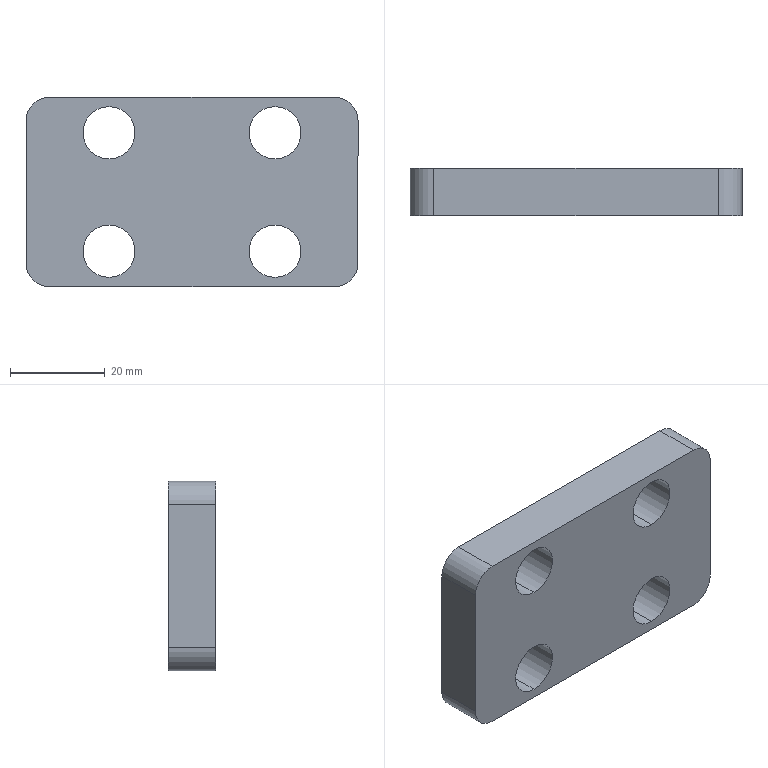Part | SolidWorks | features Extrusion 1, Fillet 1, HoleWzd 1 | 1 solid | 18 faces | box 70 x 10 x 40 mm | volume 23984 mm3 | cylinder 12 | plane 6 | commonest cylinder face diameters 11 x8 10 x4
STEP:
#1=CARTESIAN_POINT('',(-17.5,-5.,-18.));
#2=VERTEX_POINT('',#1);
#3=CARTESIAN_POINT('',(-17.5,-5.,-7.));
#4=VERTEX_POINT('',#3);
#5=CARTESIAN_POINT('',(-17.5,-5.,-12.5));
#6=DIRECTION('',(0.,1.,0.));
#7=DIRECTION('',(0.,0.,1.));
#8=AXIS2_PLACEMENT_3D('',#5,#6,#7);
#9=CIRCLE('',#8,5.5);
#10=EDGE_CURVE('',#2,#4,#9,.T.);
#11=ORIENTED_EDGE('',*,*,#10,.F.);
#12=CARTESIAN_POINT('',(-17.5,5.,-18.));
#13=VERTEX_POINT('',#12);
#14=CARTESIAN_POINT('',(-17.5,5.,-18.));
#15=DIRECTION('',(0.,1.,0.));
#16=VECTOR('',#15,1000.);
#17=LINE('',#14,#16);
#18=EDGE_CURVE('',#2,#13,#17,.T.);
#19=ORIENTED_EDGE('',*,*,#18,.T.);
#20=CARTESIAN_POINT('',(-17.5,5.,-7.));
#21=VERTEX_POINT('',#20);
#22=CARTESIAN_POINT('',(-17.5,5.,-12.5));
#23=DIRECTION('',(0.,1.,0.));
#24=DIRECTION('',(0.,0.,1.));
#25=AXIS2_PLACEMENT_3D('',#22,#23,#24);
#26=CIRCLE('',#25,5.5);
#27=EDGE_CURVE('',#13,#21,#26,.T.);
#28=ORIENTED_EDGE('',*,*,#27,.T.);
#29=CARTESIAN_POINT('',(-17.5,5.,-7.));
#30=DIRECTION('',(0.,1.,0.));
#31=VECTOR('',#30,1000.);
#32=LINE('',#29,#31);
#33=EDGE_CURVE('',#4,#21,#32,.T.);
#34=ORIENTED_EDGE('',*,*,#33,.F.);
#35=EDGE_LOOP('',(#11,#19,#28,#34));
#36=FACE_OUTER_BOUND('',#35,.T.);
#37=CARTESIAN_POINT('',(-17.5,5.,-12.5));
#38=DIRECTION('',(0.,1.,0.));
#39=DIRECTION('',(0.,0.,1.));
#40=AXIS2_PLACEMENT_3D('',#37,#38,#39);
#41=CYLINDRICAL_SURFACE('',#40,5.5);
#42=ADVANCED_FACE('',(#36),#41,.F.);
#43=CARTESIAN_POINT('',(17.5,-5.,-18.));
#44=VERTEX_POINT('',#43);
#45=CARTESIAN_POINT('',(17.5,-5.,-7.));
#46=VERTEX_POINT('',#45);
#47=CARTESIAN_POINT('',(17.5,-5.,-12.5));
#48=DIRECTION('',(0.,1.,0.));
#49=DIRECTION('',(0.,0.,1.));
#50=AXIS2_PLACEMENT_3D('',#47,#48,#49);
#51=CIRCLE('',#50,5.5);
#52=EDGE_CURVE('',#44,#46,#51,.T.);
#53=ORIENTED_EDGE('',*,*,#52,.F.);
#54=CARTESIAN_POINT('',(17.5,5.,-18.));
#55=VERTEX_POINT('',#54);
#56=CARTESIAN_POINT('',(17.5,5.,-18.));
#57=DIRECTION('',(0.,1.,0.));
#58=VECTOR('',#57,1000.);
#59=LINE('',#56,#58);
#60=EDGE_CURVE('',#44,#55,#59,.T.);
#61=ORIENTED_EDGE('',*,*,#60,.T.);
#62=CARTESIAN_POINT('',(17.5,5.,-7.));
#63=VERTEX_POINT('',#62);
#64=CARTESIAN_POINT('',(17.5,5.,-12.5));
#65=DIRECTION('',(0.,1.,0.));
#66=DIRECTION('',(0.,0.,1.));
#67=AXIS2_PLACEMENT_3D('',#64,#65,#66);
#68=CIRCLE('',#67,5.5);
#69=EDGE_CURVE('',#55,#63,#68,.T.);
#70=ORIENTED_EDGE('',*,*,#69,.T.);
#71=CARTESIAN_POINT('',(17.5,5.,-7.));
#72=DIRECTION('',(0.,1.,0.));
#73=VECTOR('',#72,1000.);
#74=LINE('',#71,#73);
#75=EDGE_CURVE('',#46,#63,#74,.T.);
#76=ORIENTED_EDGE('',*,*,#75,.F.);
#77=EDGE_LOOP('',(#53,#61,#70,#76));
#78=FACE_OUTER_BOUND('',#77,.T.);
#79=CARTESIAN_POINT('',(17.5,5.,-12.5));
#80=DIRECTION('',(0.,1.,0.));
#81=DIRECTION('',(0.,0.,1.));
#82=AXIS2_PLACEMENT_3D('',#79,#80,#81);
#83=CYLINDRICAL_SURFACE('',#82,5.5);
#84=ADVANCED_FACE('',(#78),#83,.F.);
#85=CARTESIAN_POINT('',(17.5,-5.,7.));
#86=VERTEX_POINT('',#85);
#87=CARTESIAN_POINT('',(17.5,-5.,18.));
#88=VERTEX_POINT('',#87);
#89=CARTESIAN_POINT('',(17.5,-5.,12.5));
#90=DIRECTION('',(0.,1.,0.));
#91=DIRECTION('',(0.,0.,1.));
#92=AXIS2_PLACEMENT_3D('',#89,#90,#91);
#93=CIRCLE('',#92,5.5);
#94=EDGE_CURVE('',#86,#88,#93,.T.);
#95=ORIENTED_EDGE('',*,*,#94,.F.);
#96=CARTESIAN_POINT('',(17.5,5.,7.));
#97=VERTEX_POINT('',#96);
#98=CARTESIAN_POINT('',(17.5,5.,7.));
#99=DIRECTION('',(0.,1.,0.));
#100=VECTOR('',#99,1000.);
#101=LINE('',#98,#100);
#102=EDGE_CURVE('',#86,#97,#101,.T.);
#103=ORIENTED_EDGE('',*,*,#102,.T.);
#104=CARTESIAN_POINT('',(17.5,5.,18.));
#105=VERTEX_POINT('',#104);
#106=CARTESIAN_POINT('',(17.5,5.,12.5));
#107=DIRECTION('',(0.,1.,0.));
#108=DIRECTION('',(0.,0.,1.));
#109=AXIS2_PLACEMENT_3D('',#106,#107,#108);
#110=CIRCLE('',#109,5.5);
#111=EDGE_CURVE('',#97,#105,#110,.T.);
#112=ORIENTED_EDGE('',*,*,#111,.T.);
#113=CARTESIAN_POINT('',(17.5,5.,18.));
#114=DIRECTION('',(0.,1.,0.));
#115=VECTOR('',#114,1000.);
#116=LINE('',#113,#115);
#117=EDGE_CURVE('',#88,#105,#116,.T.);
#118=ORIENTED_EDGE('',*,*,#117,.F.);
#119=EDGE_LOOP('',(#95,#103,#112,#118));
#120=FACE_OUTER_BOUND('',#119,.T.);
#121=CARTESIAN_POINT('',(17.5,5.,12.5));
#122=DIRECTION('',(0.,1.,0.));
#123=DIRECTION('',(0.,0.,1.));
#124=AXIS2_PLACEMENT_3D('',#121,#122,#123);
#125=CYLINDRICAL_SURFACE('',#124,5.5);
#126=ADVANCED_FACE('',(#120),#125,.F.);
#127=CARTESIAN_POINT('',(-17.5,-5.,7.));
#128=VERTEX_POINT('',#127);
#129=CARTESIAN_POINT('',(-17.5,-5.,18.));
#130=VERTEX_POINT('',#129);
#131=CARTESIAN_POINT('',(-17.5,-5.,12.5));
#132=DIRECTION('',(0.,1.,0.));
#133=DIRECTION('',(0.,0.,1.));
#134=AXIS2_PLACEMENT_3D('',#131,#132,#133);
#135=CIRCLE('',#134,5.5);
#136=EDGE_CURVE('',#128,#130,#135,.T.);
#137=ORIENTED_EDGE('',*,*,#136,.F.);
#138=CARTESIAN_POINT('',(-17.5,5.,7.));
#139=VERTEX_POINT('',#138);
#140=CARTESIAN_POINT('',(-17.5,5.,7.));
#141=DIRECTION('',(0.,1.,0.));
#142=VECTOR('',#141,1000.);
#143=LINE('',#140,#142);
#144=EDGE_CURVE('',#128,#139,#143,.T.);
#145=ORIENTED_EDGE('',*,*,#144,.T.);
#146=CARTESIAN_POINT('',(-17.5,5.,18.));
#147=VERTEX_POINT('',#146);
#148=CARTESIAN_POINT('',(-17.5,5.,12.5));
#149=DIRECTION('',(0.,1.,0.));
#150=DIRECTION('',(0.,0.,1.));
#151=AXIS2_PLACEMENT_3D('',#148,#149,#150);
#152=CIRCLE('',#151,5.5);
#153=EDGE_CURVE('',#139,#147,#152,.T.);
#154=ORIENTED_EDGE('',*,*,#153,.T.);
#155=CARTESIAN_POINT('',(-17.5,5.,18.));
#156=DIRECTION('',(0.,1.,0.));
#157=VECTOR('',#156,1000.);
#158=LINE('',#155,#157);
#159=EDGE_CURVE('',#130,#147,#158,.T.);
#160=ORIENTED_EDGE('',*,*,#159,.F.);
#161=EDGE_LOOP('',(#137,#145,#154,#160));
#162=FACE_OUTER_BOUND('',#161,.T.);
#163=CARTESIAN_POINT('',(-17.5,5.,12.5));
#164=DIRECTION('',(0.,1.,0.));
#165=DIRECTION('',(0.,0.,1.));
#166=AXIS2_PLACEMENT_3D('',#163,#164,#165);
#167=CYLINDRICAL_SURFACE('',#166,5.5);
#168=ADVANCED_FACE('',(#162),#167,.F.);
#169=CARTESIAN_POINT('',(35.,5.,15.));
#170=VERTEX_POINT('',#169);
#171=CARTESIAN_POINT('',(35.,5.,-15.));
#172=VERTEX_POINT('',#171);
#173=CARTESIAN_POINT('',(35.,5.,-20.));
#174=DIRECTION('',(0.,0.,-1.));
#175=VECTOR('',#174,1000.);
#176=LINE('',#173,#175);
#177=EDGE_CURVE('',#170,#172,#176,.T.);
#178=ORIENTED_EDGE('',*,*,#177,.F.);
#179=CARTESIAN_POINT('',(35.,-5.,15.));
#180=VERTEX_POINT('',#179);
#181=CARTESIAN_POINT('',(35.,5.,15.));
#182=DIRECTION('',(0.,-1.,0.));
#183=VECTOR('',#182,1000.);
#184=LINE('',#181,#183);
#185=EDGE_CURVE('',#170,#180,#184,.T.);
#186=ORIENTED_EDGE('',*,*,#185,.T.);
#187=CARTESIAN_POINT('',(35.,-5.,-15.));
#188=VERTEX_POINT('',#187);
#189=CARTESIAN_POINT('',(35.,-5.,-20.));
#190=DIRECTION('',(0.,0.,-1.));
#191=VECTOR('',#190,1000.);
#192=LINE('',#189,#191);
#193=EDGE_CURVE('',#180,#188,#192,.T.);
#194=ORIENTED_EDGE('',*,*,#193,.T.);
#195=CARTESIAN_POINT('',(35.,5.,-15.));
#196=DIRECTION('',(0.,1.,0.));
#197=VECTOR('',#196,1000.);
#198=LINE('',#195,#197);
#199=EDGE_CURVE('',#188,#172,#198,.T.);
#200=ORIENTED_EDGE('',*,*,#199,.T.);
#201=EDGE_LOOP('',(#178,#186,#194,#200));
#202=FACE_OUTER_BOUND('',#201,.T.);
#203=CARTESIAN_POINT('',(35.,5.,-20.));
#204=DIRECTION('',(-1.,0.,0.));
#205=DIRECTION('',(0.,0.,1.));
#206=AXIS2_PLACEMENT_3D('',#203,#204,#205);
#207=PLANE('',#206);
#208=ADVANCED_FACE('',(#202),#207,.F.);
#209=CARTESIAN_POINT('',(30.,-5.,-20.));
#210=VERTEX_POINT('',#209);
#211=CARTESIAN_POINT('',(-30.,-5.,-20.));
#212=VERTEX_POINT('',#211);
#213=CARTESIAN_POINT('',(-35.,-5.,-20.));
#214=DIRECTION('',(-1.,0.,0.));
#215=VECTOR('',#214,1000.);
#216=LINE('',#213,#215);
#217=EDGE_CURVE('',#210,#212,#216,.T.);
#218=ORIENTED_EDGE('',*,*,#217,.T.);
#219=CARTESIAN_POINT('',(-30.,5.,-20.));
#220=VERTEX_POINT('',#219);
#221=CARTESIAN_POINT('',(-30.,5.,-20.));
#222=DIRECTION('',(0.,1.,0.));
#223=VECTOR('',#222,1000.);
#224=LINE('',#221,#223);
#225=EDGE_CURVE('',#212,#220,#224,.T.);
#226=ORIENTED_EDGE('',*,*,#225,.T.);
#227=CARTESIAN_POINT('',(30.,5.,-20.));
#228=VERTEX_POINT('',#227);
#229=CARTESIAN_POINT('',(-35.,5.,-20.));
#230=DIRECTION('',(-1.,0.,0.));
#231=VECTOR('',#230,1000.);
#232=LINE('',#229,#231);
#233=EDGE_CURVE('',#228,#220,#232,.T.);
#234=ORIENTED_EDGE('',*,*,#233,.F.);
#235=CARTESIAN_POINT('',(30.,5.,-20.));
#236=DIRECTION('',(0.,-1.,0.));
#237=VECTOR('',#236,1000.);
#238=LINE('',#235,#237);
#239=EDGE_CURVE('',#228,#210,#238,.T.);
#240=ORIENTED_EDGE('',*,*,#239,.T.);
#241=EDGE_LOOP('',(#218,#226,#234,#240));
#242=FACE_OUTER_BOUND('',#241,.T.);
#243=CARTESIAN_POINT('',(-35.,5.,-20.));
#244=DIRECTION('',(0.,0.,1.));
#245=DIRECTION('',(1.,0.,0.));
#246=AXIS2_PLACEMENT_3D('',#243,#244,#245);
#247=PLANE('',#246);
#248=ADVANCED_FACE('',(#242),#247,.F.);
#249=CARTESIAN_POINT('',(-35.,5.,-15.));
#250=VERTEX_POINT('',#249);
#251=CARTESIAN_POINT('',(-35.,5.,15.));
#252=VERTEX_POINT('',#251);
#253=CARTESIAN_POINT('',(-35.,5.,-20.));
#254=DIRECTION('',(0.,0.,1.));
#255=VECTOR('',#254,1000.);
#256=LINE('',#253,#255);
#257=EDGE_CURVE('',#250,#252,#256,.T.);
#258=ORIENTED_EDGE('',*,*,#257,.F.);
#259=CARTESIAN_POINT('',(-35.,-5.,-15.));
#260=VERTEX_POINT('',#259);
#261=CARTESIAN_POINT('',(-35.,5.,-15.));
#262=DIRECTION('',(0.,-1.,0.));
#263=VECTOR('',#262,1000.);
#264=LINE('',#261,#263);
#265=EDGE_CURVE('',#250,#260,#264,.T.);
#266=ORIENTED_EDGE('',*,*,#265,.T.);
#267=CARTESIAN_POINT('',(-35.,-5.,15.));
#268=VERTEX_POINT('',#267);
#269=CARTESIAN_POINT('',(-35.,-5.,-20.));
#270=DIRECTION('',(0.,0.,1.));
#271=VECTOR('',#270,1000.);
#272=LINE('',#269,#271);
#273=EDGE_CURVE('',#260,#268,#272,.T.);
#274=ORIENTED_EDGE('',*,*,#273,.T.);
#275=CARTESIAN_POINT('',(-35.,5.,15.));
#276=DIRECTION('',(0.,1.,0.));
#277=VECTOR('',#276,1000.);
#278=LINE('',#275,#277);
#279=EDGE_CURVE('',#268,#252,#278,.T.);
#280=ORIENTED_EDGE('',*,*,#279,.T.);
#281=EDGE_LOOP('',(#258,#266,#274,#280));
#282=FACE_OUTER_BOUND('',#281,.T.);
#283=CARTESIAN_POINT('',(-35.,5.,-20.));
#284=DIRECTION('',(1.,0.,0.));
#285=DIRECTION('',(0.,0.,-1.));
#286=AXIS2_PLACEMENT_3D('',#283,#284,#285);
#287=PLANE('',#286);
#288=ADVANCED_FACE('',(#282),#287,.F.);
#289=CARTESIAN_POINT('',(-30.,-5.,20.));
#290=VERTEX_POINT('',#289);
#291=CARTESIAN_POINT('',(30.,-5.,20.));
#292=VERTEX_POINT('',#291);
#293=CARTESIAN_POINT('',(-35.,-5.,20.));
#294=DIRECTION('',(1.,0.,0.));
#295=VECTOR('',#294,1000.);
#296=LINE('',#293,#295);
#297=EDGE_CURVE('',#290,#292,#296,.T.);
#298=ORIENTED_EDGE('',*,*,#297,.T.);
#299=CARTESIAN_POINT('',(30.,5.,20.));
#300=VERTEX_POINT('',#299);
#301=CARTESIAN_POINT('',(30.,5.,20.));
#302=DIRECTION('',(0.,1.,0.));
#303=VECTOR('',#302,1000.);
#304=LINE('',#301,#303);
#305=EDGE_CURVE('',#292,#300,#304,.T.);
#306=ORIENTED_EDGE('',*,*,#305,.T.);
#307=CARTESIAN_POINT('',(-30.,5.,20.));
#308=VERTEX_POINT('',#307);
#309=CARTESIAN_POINT('',(-35.,5.,20.));
#310=DIRECTION('',(1.,0.,0.));
#311=VECTOR('',#310,1000.);
#312=LINE('',#309,#311);
#313=EDGE_CURVE('',#308,#300,#312,.T.);
#314=ORIENTED_EDGE('',*,*,#313,.F.);
#315=CARTESIAN_POINT('',(-30.,5.,20.));
#316=DIRECTION('',(0.,-1.,0.));
#317=VECTOR('',#316,1000.);
#318=LINE('',#315,#317);
#319=EDGE_CURVE('',#308,#290,#318,.T.);
#320=ORIENTED_EDGE('',*,*,#319,.T.);
#321=EDGE_LOOP('',(#298,#306,#314,#320));
#322=FACE_OUTER_BOUND('',#321,.T.);
#323=CARTESIAN_POINT('',(-35.,5.,20.));
#324=DIRECTION('',(0.,0.,-1.));
#325=DIRECTION('',(-1.,0.,0.));
#326=AXIS2_PLACEMENT_3D('',#323,#324,#325);
#327=PLANE('',#326);
#328=ADVANCED_FACE('',(#322),#327,.F.);
#329=CARTESIAN_POINT('',(-17.5,5.,-12.5));
#330=DIRECTION('',(0.,1.,0.));
#331=DIRECTION('',(0.,0.,1.));
#332=AXIS2_PLACEMENT_3D('',#329,#330,#331);
#333=CIRCLE('',#332,5.5);
#334=EDGE_CURVE('',#21,#13,#333,.T.);
#335=ORIENTED_EDGE('',*,*,#334,.F.);
#336=ORIENTED_EDGE('',*,*,#27,.F.);
#337=EDGE_LOOP('',(#335,#336));
#338=FACE_BOUND('',#337,.T.);
#339=CARTESIAN_POINT('',(17.5,5.,-12.5));
#340=DIRECTION('',(0.,1.,0.));
#341=DIRECTION('',(0.,0.,1.));
#342=AXIS2_PLACEMENT_3D('',#339,#340,#341);
#343=CIRCLE('',#342,5.5);
#344=EDGE_CURVE('',#63,#55,#343,.T.);
#345=ORIENTED_EDGE('',*,*,#344,.F.);
#346=ORIENTED_EDGE('',*,*,#69,.F.);
#347=EDGE_LOOP('',(#345,#346));
#348=FACE_BOUND('',#347,.T.);
#349=CARTESIAN_POINT('',(17.5,5.,12.5));
#350=DIRECTION('',(0.,1.,0.));
#351=DIRECTION('',(0.,0.,1.));
#352=AXIS2_PLACEMENT_3D('',#349,#350,#351);
#353=CIRCLE('',#352,5.5);
#354=EDGE_CURVE('',#105,#97,#353,.T.);
#355=ORIENTED_EDGE('',*,*,#354,.F.);
#356=ORIENTED_EDGE('',*,*,#111,.F.);
#357=EDGE_LOOP('',(#355,#356));
#358=FACE_BOUND('',#357,.T.);
#359=CARTESIAN_POINT('',(-17.5,5.,12.5));
#360=DIRECTION('',(0.,1.,0.));
#361=DIRECTION('',(0.,0.,1.));
#362=AXIS2_PLACEMENT_3D('',#359,#360,#361);
#363=CIRCLE('',#362,5.5);
#364=EDGE_CURVE('',#147,#139,#363,.T.);
#365=ORIENTED_EDGE('',*,*,#364,.F.);
#366=ORIENTED_EDGE('',*,*,#153,.F.);
#367=EDGE_LOOP('',(#365,#366));
#368=FACE_BOUND('',#367,.T.);
#369=ORIENTED_EDGE('',*,*,#313,.T.);
#370=CARTESIAN_POINT('',(30.,5.,15.));
#371=DIRECTION('',(0.,1.,0.));
#372=DIRECTION('',(0.,0.,1.));
#373=AXIS2_PLACEMENT_3D('',#370,#371,#372);
#374=CIRCLE('',#373,5.);
#375=EDGE_CURVE('',#300,#170,#374,.T.);
#376=ORIENTED_EDGE('',*,*,#375,.T.);
#377=ORIENTED_EDGE('',*,*,#177,.T.);
#378=CARTESIAN_POINT('',(30.,5.,-15.));
#379=DIRECTION('',(0.,1.,0.));
#380=DIRECTION('',(0.,0.,1.));
#381=AXIS2_PLACEMENT_3D('',#378,#379,#380);
#382=CIRCLE('',#381,5.);
#383=EDGE_CURVE('',#172,#228,#382,.T.);
#384=ORIENTED_EDGE('',*,*,#383,.T.);
#385=ORIENTED_EDGE('',*,*,#233,.T.);
#386=CARTESIAN_POINT('',(-30.,5.,-15.));
#387=DIRECTION('',(0.,1.,0.));
#388=DIRECTION('',(0.,0.,1.));
#389=AXIS2_PLACEMENT_3D('',#386,#387,#388);
#390=CIRCLE('',#389,5.);
#391=EDGE_CURVE('',#220,#250,#390,.T.);
#392=ORIENTED_EDGE('',*,*,#391,.T.);
#393=ORIENTED_EDGE('',*,*,#257,.T.);
#394=CARTESIAN_POINT('',(-30.,5.,15.));
#395=DIRECTION('',(0.,1.,0.));
#396=DIRECTION('',(0.,0.,1.));
#397=AXIS2_PLACEMENT_3D('',#394,#395,#396);
#398=CIRCLE('',#397,5.);
#399=EDGE_CURVE('',#252,#308,#398,.T.);
#400=ORIENTED_EDGE('',*,*,#399,.T.);
#401=EDGE_LOOP('',(#369,#376,#377,#384,#385,#392,#393,#400));
#402=FACE_OUTER_BOUND('',#401,.T.);
#403=CARTESIAN_POINT('',(0.,5.,0.));
#404=DIRECTION('',(0.,1.,0.));
#405=DIRECTION('',(0.,0.,1.));
#406=AXIS2_PLACEMENT_3D('',#403,#404,#405);
#407=PLANE('',#406);
#408=ADVANCED_FACE('',(#338,#348,#358,#368,#402),#407,.T.);
#409=CARTESIAN_POINT('',(-17.5,-5.,-12.5));
#410=DIRECTION('',(0.,1.,0.));
#411=DIRECTION('',(0.,0.,1.));
#412=AXIS2_PLACEMENT_3D('',#409,#410,#411);
#413=CIRCLE('',#412,5.5);
#414=EDGE_CURVE('',#4,#2,#413,.T.);
#415=ORIENTED_EDGE('',*,*,#414,.T.);
#416=ORIENTED_EDGE('',*,*,#10,.T.);
#417=EDGE_LOOP('',(#415,#416));
#418=FACE_BOUND('',#417,.T.);
#419=CARTESIAN_POINT('',(17.5,-5.,-12.5));
#420=DIRECTION('',(0.,1.,0.));
#421=DIRECTION('',(0.,0.,1.));
#422=AXIS2_PLACEMENT_3D('',#419,#420,#421);
#423=CIRCLE('',#422,5.5);
#424=EDGE_CURVE('',#46,#44,#423,.T.);
#425=ORIENTED_EDGE('',*,*,#424,.T.);
#426=ORIENTED_EDGE('',*,*,#52,.T.);
#427=EDGE_LOOP('',(#425,#426));
#428=FACE_BOUND('',#427,.T.);
#429=CARTESIAN_POINT('',(17.5,-5.,12.5));
#430=DIRECTION('',(0.,1.,0.));
#431=DIRECTION('',(0.,0.,1.));
#432=AXIS2_PLACEMENT_3D('',#429,#430,#431);
#433=CIRCLE('',#432,5.5);
#434=EDGE_CURVE('',#88,#86,#433,.T.);
#435=ORIENTED_EDGE('',*,*,#434,.T.);
#436=ORIENTED_EDGE('',*,*,#94,.T.);
#437=EDGE_LOOP('',(#435,#436));
#438=FACE_BOUND('',#437,.T.);
#439=CARTESIAN_POINT('',(-17.5,-5.,12.5));
#440=DIRECTION('',(0.,1.,0.));
#441=DIRECTION('',(0.,0.,1.));
#442=AXIS2_PLACEMENT_3D('',#439,#440,#441);
#443=CIRCLE('',#442,5.5);
#444=EDGE_CURVE('',#130,#128,#443,.T.);
#445=ORIENTED_EDGE('',*,*,#444,.T.);
#446=ORIENTED_EDGE('',*,*,#136,.T.);
#447=EDGE_LOOP('',(#445,#446));
#448=FACE_BOUND('',#447,.T.);
#449=ORIENTED_EDGE('',*,*,#193,.F.);
#450=CARTESIAN_POINT('',(30.,-5.,15.));
#451=DIRECTION('',(0.,-1.,0.));
#452=DIRECTION('',(0.,0.,1.));
#453=AXIS2_PLACEMENT_3D('',#450,#451,#452);
#454=CIRCLE('',#453,5.);
#455=EDGE_CURVE('',#180,#292,#454,.T.);
#456=ORIENTED_EDGE('',*,*,#455,.T.);
#457=ORIENTED_EDGE('',*,*,#297,.F.);
#458=CARTESIAN_POINT('',(-30.,-5.,15.));
#459=DIRECTION('',(0.,-1.,0.));
#460=DIRECTION('',(0.,0.,1.));
#461=AXIS2_PLACEMENT_3D('',#458,#459,#460);
#462=CIRCLE('',#461,5.);
#463=EDGE_CURVE('',#290,#268,#462,.T.);
#464=ORIENTED_EDGE('',*,*,#463,.T.);
#465=ORIENTED_EDGE('',*,*,#273,.F.);
#466=CARTESIAN_POINT('',(-30.,-5.,-15.));
#467=DIRECTION('',(0.,-1.,0.));
#468=DIRECTION('',(0.,0.,1.));
#469=AXIS2_PLACEMENT_3D('',#466,#467,#468);
#470=CIRCLE('',#469,5.);
#471=EDGE_CURVE('',#260,#212,#470,.T.);
#472=ORIENTED_EDGE('',*,*,#471,.T.);
#473=ORIENTED_EDGE('',*,*,#217,.F.);
#474=CARTESIAN_POINT('',(30.,-5.,-15.));
#475=DIRECTION('',(0.,-1.,0.));
#476=DIRECTION('',(0.,0.,1.));
#477=AXIS2_PLACEMENT_3D('',#474,#475,#476);
#478=CIRCLE('',#477,5.);
#479=EDGE_CURVE('',#210,#188,#478,.T.);
#480=ORIENTED_EDGE('',*,*,#479,.T.);
#481=EDGE_LOOP('',(#449,#456,#457,#464,#465,#472,#473,#480));
#482=FACE_OUTER_BOUND('',#481,.T.);
#483=CARTESIAN_POINT('',(0.,-5.,0.));
#484=DIRECTION('',(0.,1.,0.));
#485=DIRECTION('',(0.,0.,1.));
#486=AXIS2_PLACEMENT_3D('',#483,#484,#485);
#487=PLANE('',#486);
#488=ADVANCED_FACE('',(#418,#428,#438,#448,#482),#487,.F.);
#489=ORIENTED_EDGE('',*,*,#144,.F.);
#490=ORIENTED_EDGE('',*,*,#444,.F.);
#491=ORIENTED_EDGE('',*,*,#159,.T.);
#492=ORIENTED_EDGE('',*,*,#364,.T.);
#493=EDGE_LOOP('',(#489,#490,#491,#492));
#494=FACE_OUTER_BOUND('',#493,.T.);
#495=CARTESIAN_POINT('',(-17.5,5.,12.5));
#496=DIRECTION('',(0.,1.,0.));
#497=DIRECTION('',(0.,0.,1.));
#498=AXIS2_PLACEMENT_3D('',#495,#496,#497);
#499=CYLINDRICAL_SURFACE('',#498,5.5);
#500=ADVANCED_FACE('',(#494),#499,.F.);
#501=ORIENTED_EDGE('',*,*,#102,.F.);
#502=ORIENTED_EDGE('',*,*,#434,.F.);
#503=ORIENTED_EDGE('',*,*,#117,.T.);
#504=ORIENTED_EDGE('',*,*,#354,.T.);
#505=EDGE_LOOP('',(#501,#502,#503,#504));
#506=FACE_OUTER_BOUND('',#505,.T.);
#507=CARTESIAN_POINT('',(17.5,5.,12.5));
#508=DIRECTION('',(0.,1.,0.));
#509=DIRECTION('',(0.,0.,1.));
#510=AXIS2_PLACEMENT_3D('',#507,#508,#509);
#511=CYLINDRICAL_SURFACE('',#510,5.5);
#512=ADVANCED_FACE('',(#506),#511,.F.);
#513=ORIENTED_EDGE('',*,*,#60,.F.);
#514=ORIENTED_EDGE('',*,*,#424,.F.);
#515=ORIENTED_EDGE('',*,*,#75,.T.);
#516=ORIENTED_EDGE('',*,*,#344,.T.);
#517=EDGE_LOOP('',(#513,#514,#515,#516));
#518=FACE_OUTER_BOUND('',#517,.T.);
#519=CARTESIAN_POINT('',(17.5,5.,-12.5));
#520=DIRECTION('',(0.,1.,0.));
#521=DIRECTION('',(0.,0.,1.));
#522=AXIS2_PLACEMENT_3D('',#519,#520,#521);
#523=CYLINDRICAL_SURFACE('',#522,5.5);
#524=ADVANCED_FACE('',(#518),#523,.F.);
#525=ORIENTED_EDGE('',*,*,#18,.F.);
#526=ORIENTED_EDGE('',*,*,#414,.F.);
#527=ORIENTED_EDGE('',*,*,#33,.T.);
#528=ORIENTED_EDGE('',*,*,#334,.T.);
#529=EDGE_LOOP('',(#525,#526,#527,#528));
#530=FACE_OUTER_BOUND('',#529,.T.);
#531=CARTESIAN_POINT('',(-17.5,5.,-12.5));
#532=DIRECTION('',(0.,1.,0.));
#533=DIRECTION('',(0.,0.,1.));
#534=AXIS2_PLACEMENT_3D('',#531,#532,#533);
#535=CYLINDRICAL_SURFACE('',#534,5.5);
#536=ADVANCED_FACE('',(#530),#535,.F.);
#537=ORIENTED_EDGE('',*,*,#375,.F.);
#538=ORIENTED_EDGE('',*,*,#305,.F.);
#539=ORIENTED_EDGE('',*,*,#455,.F.);
#540=ORIENTED_EDGE('',*,*,#185,.F.);
#541=EDGE_LOOP('',(#537,#538,#539,#540));
#542=FACE_OUTER_BOUND('',#541,.T.);
#543=CARTESIAN_POINT('',(30.,5.,15.));
#544=DIRECTION('',(0.,-1.,0.));
#545=DIRECTION('',(0.,0.,-1.));
#546=AXIS2_PLACEMENT_3D('',#543,#544,#545);
#547=CYLINDRICAL_SURFACE('',#546,5.);
#548=ADVANCED_FACE('',(#542),#547,.T.);
#549=ORIENTED_EDGE('',*,*,#391,.F.);
#550=ORIENTED_EDGE('',*,*,#225,.F.);
#551=ORIENTED_EDGE('',*,*,#471,.F.);
#552=ORIENTED_EDGE('',*,*,#265,.F.);
#553=EDGE_LOOP('',(#549,#550,#551,#552));
#554=FACE_OUTER_BOUND('',#553,.T.);
#555=CARTESIAN_POINT('',(-30.,5.,-15.));
#556=DIRECTION('',(0.,-1.,0.));
#557=DIRECTION('',(0.,0.,-1.));
#558=AXIS2_PLACEMENT_3D('',#555,#556,#557);
#559=CYLINDRICAL_SURFACE('',#558,5.);
#560=ADVANCED_FACE('',(#554),#559,.T.);
#561=ORIENTED_EDGE('',*,*,#383,.F.);
#562=ORIENTED_EDGE('',*,*,#199,.F.);
#563=ORIENTED_EDGE('',*,*,#479,.F.);
#564=ORIENTED_EDGE('',*,*,#239,.F.);
#565=EDGE_LOOP('',(#561,#562,#563,#564));
#566=FACE_OUTER_BOUND('',#565,.T.);
#567=CARTESIAN_POINT('',(30.,5.,-15.));
#568=DIRECTION('',(0.,-1.,0.));
#569=DIRECTION('',(0.,0.,-1.));
#570=AXIS2_PLACEMENT_3D('',#567,#568,#569);
#571=CYLINDRICAL_SURFACE('',#570,5.);
#572=ADVANCED_FACE('',(#566),#571,.T.);
#573=ORIENTED_EDGE('',*,*,#399,.F.);
#574=ORIENTED_EDGE('',*,*,#279,.F.);
#575=ORIENTED_EDGE('',*,*,#463,.F.);
#576=ORIENTED_EDGE('',*,*,#319,.F.);
#577=EDGE_LOOP('',(#573,#574,#575,#576));
#578=FACE_OUTER_BOUND('',#577,.T.);
#579=CARTESIAN_POINT('',(-30.,5.,15.));
#580=DIRECTION('',(0.,-1.,0.));
#581=DIRECTION('',(0.,0.,-1.));
#582=AXIS2_PLACEMENT_3D('',#579,#580,#581);
#583=CYLINDRICAL_SURFACE('',#582,5.);
#584=ADVANCED_FACE('',(#578),#583,.T.);
#585=CLOSED_SHELL('',(#42,#84,#126,#168,#208,#248,#288,#328,#408,#488,#500,#512,#524,#536,#548,#560,#572,#584));
#586=MANIFOLD_SOLID_BREP('',#585);
#587=CARTESIAN_POINT('',(0.,0.,0.));
#588=DIRECTION('',(0.,0.,1.));
#589=DIRECTION('',(1.,0.,0.));
#590=AXIS2_PLACEMENT_3D('',#587,#588,#589);
#591=(LENGTH_UNIT()NAMED_UNIT(*)SI_UNIT(.MILLI.,.METRE.));
#592=UNCERTAINTY_MEASURE_WITH_UNIT(LENGTH_MEASURE(0.00001),#591,'','');
#593=(NAMED_UNIT(*)PLANE_ANGLE_UNIT()SI_UNIT($,.RADIAN.));
#594=(NAMED_UNIT(*)SI_UNIT($,.STERADIAN.)SOLID_ANGLE_UNIT());
#595=(GEOMETRIC_REPRESENTATION_CONTEXT(3)GLOBAL_UNCERTAINTY_ASSIGNED_CONTEXT((#592))GLOBAL_UNIT_ASSIGNED_CONTEXT((#591,#593,#594))REPRESENTATION_CONTEXT('',''));
#596=ADVANCED_BREP_SHAPE_REPRESENTATION('',(#586,#590),#595);